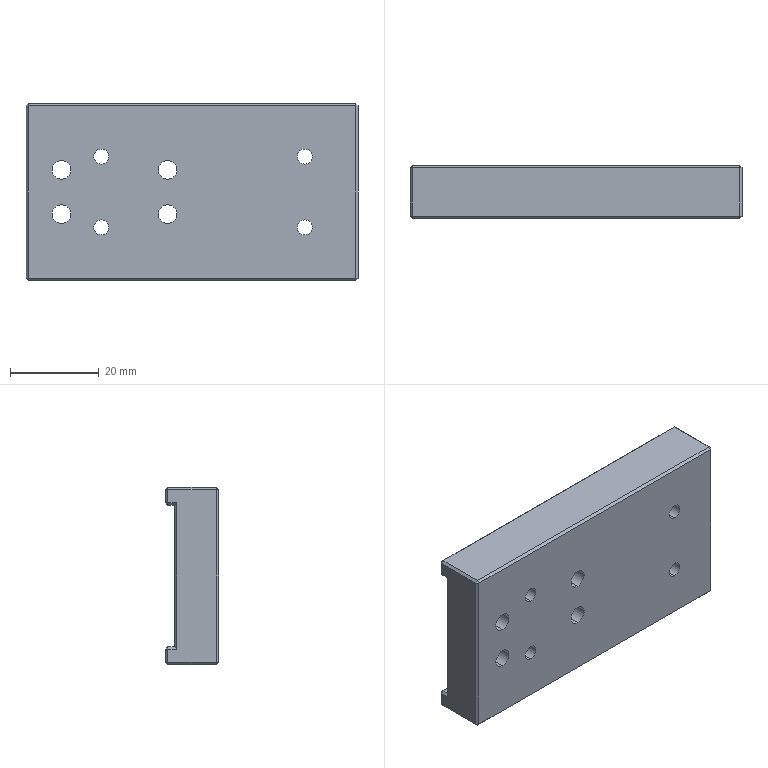Part | STEP file | ND25021-01-JDKM-34-TL | 1 solid | 72 faces | box 75 x 12 x 40 mm | volume 29872 mm3 | plane 48 | cylinder 24 | commonest cylinder face diameters 3.4 x8 4.2 x8 6.5 x8